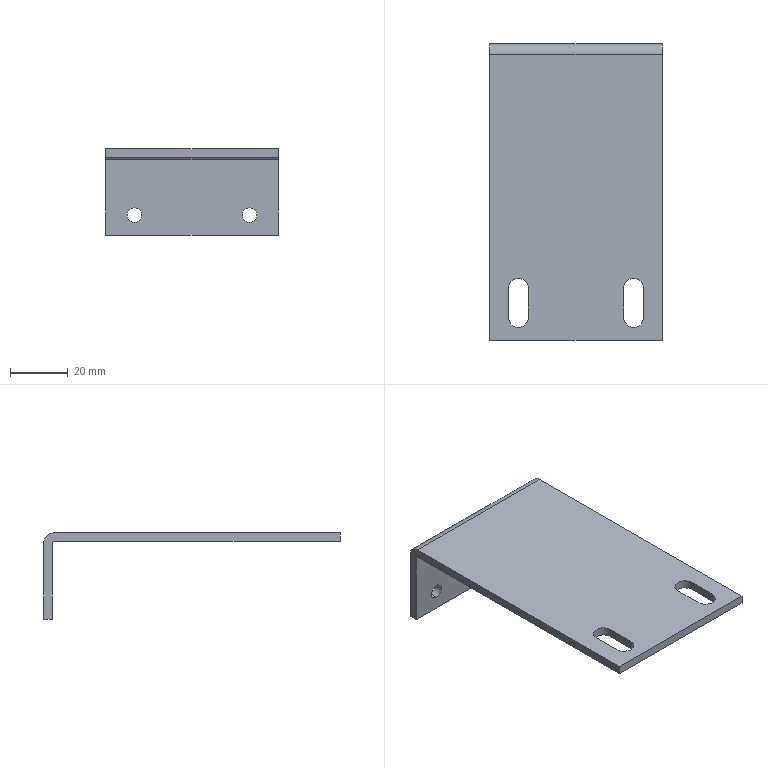Part | STEP file | PN_0005_bracket | 1 solid | 22 faces | box 60 x 103 x 30 mm | volume 22458 mm3 | plane 12 | cylinder 10 | commonest cylinder face diameters 5 x4 7 x4 1.473 x1 7.473 x1